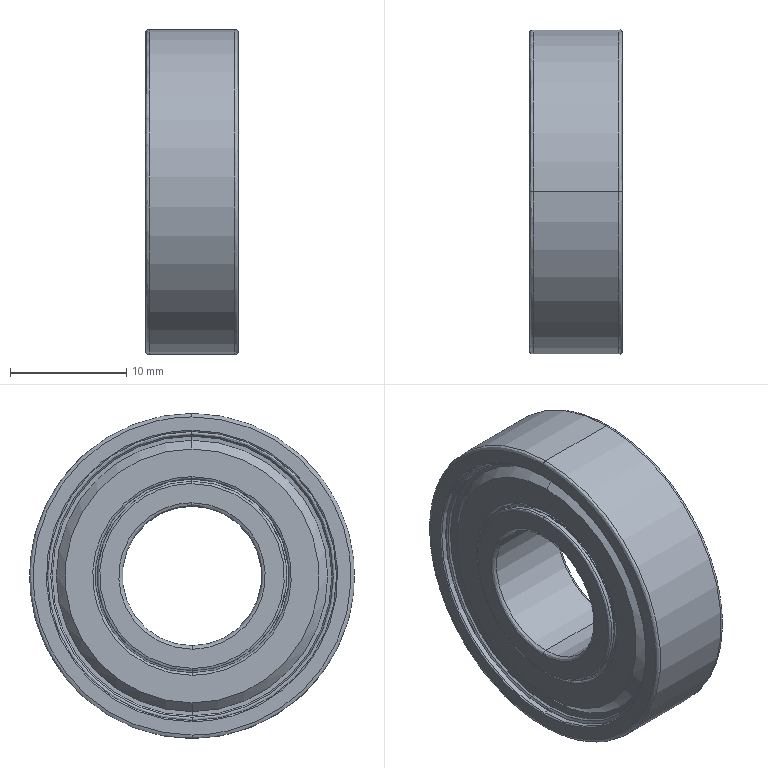Part | SolidWorks | features BaseBody 1 | 1 solid | 128 faces | box 8 x 28 x 28 mm | volume 3203 mm3 | spline 48 | cone 36 | cylinder 32 | plane 12 | commonest cylinder face diameters 15.5 x4 16.3 x4 16.7 x4 17.1 x4 17.5 x4 23.5 x4